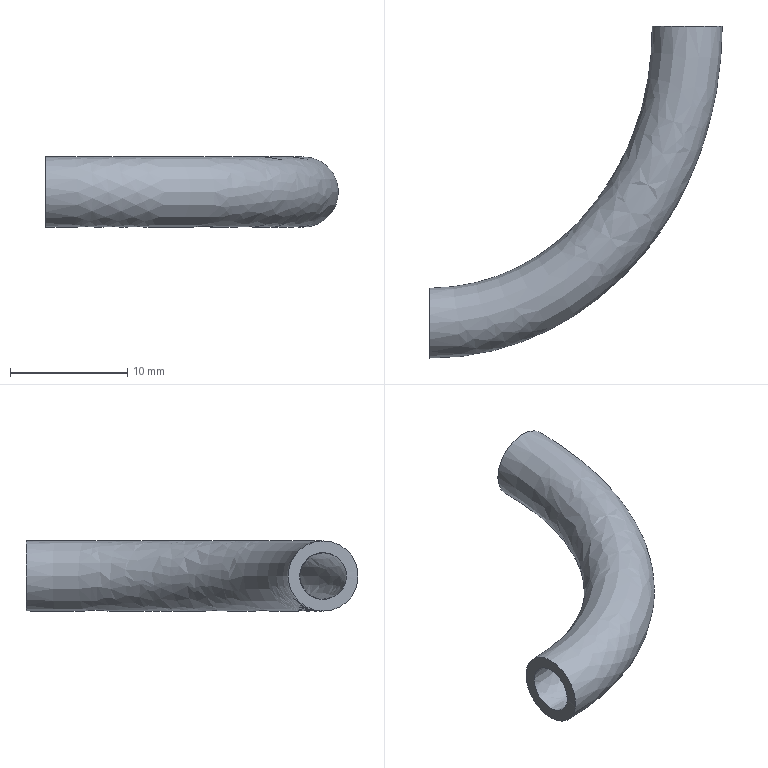Part | NX | features solid 2 | 1 solid | 4 faces | box 25.009 x 28.387 x 6 mm | volume 585.461 mm3 | plane 2 | spline 2